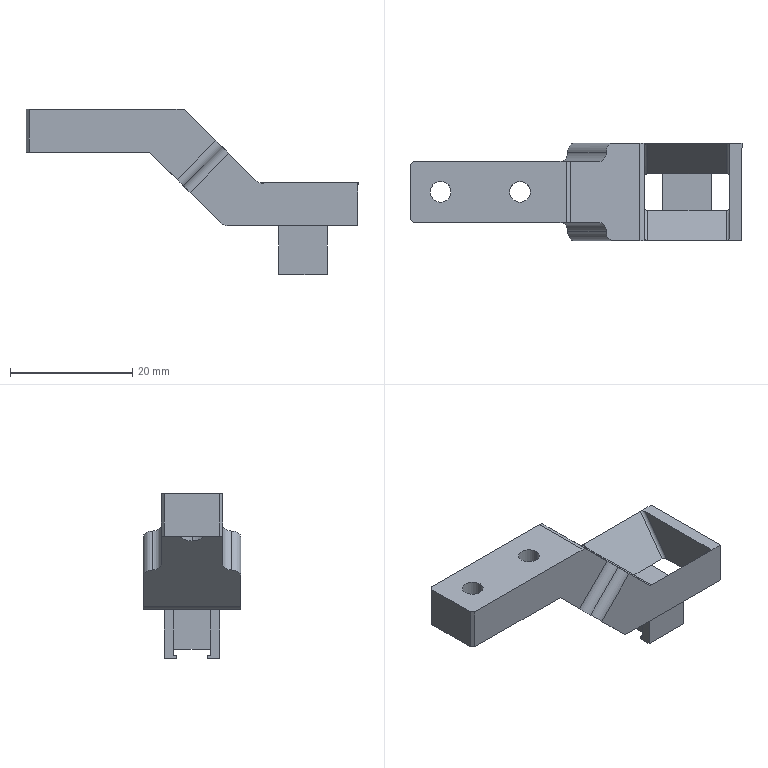NC program | NX | posted with a generic post | part box 54.3 x 16 x 27 mm
Lines 578 to 2261 of 2261, first 1553 of 1680 lines:
(ZLEVEL_PROFILE_COPY_1 , TOOL : D4R0.2)
N1124 T05 M6
N1126 G54
N1128 G17 G0 G90 X3.006 Y-8.122 S9500 M3
N1130 G43 Z30. H5
N1132 Z-4.367
N1134 G94 G1 Z-5.867 F800.
N1136 X3.412 Y-7.653
N1138 G3 X3.488 Y-7.26 R0.4
N1140 G1 X3.424 Y-7.076 F2000.
N1142 X3.414 Y-7.041
N1144 X3.408 Y-7.007
N1146 X3.344 Y-7.003
N1148 X2.618 Y-6.999
N1150 X2.546 Z-5.939
N1152 X3.334 Y-7.007
N1154 X3.344 Y-7.015
N1156 X3.374 Y-7.116
N1158 G3 X3.697 Y-7.893 R3.536
N1160 G1 X3.738 Y-8.01 Z-5.957
N1162 X3.783 Y-8.126 Z-5.975
N1164 X3.834 Y-8.237 Z-5.993
N1166 X3.895 Y-8.343 Z-6.011
N1168 G2 X3.272 Y-7.007 R4.174
N1170 G1 X2.475 Y-6.999
N1172 X2.403 Z-6.083
N1174 X3.062 Y-7.001
N1176 X3.21 Y-7.008
N1178 G3 X4.138 Y-8.696 R3.428
N1180 G1 X4.203 Y-8.795 Z-6.107
N1182 X4.274 Y-8.888 Z-6.131
N1184 X4.356 Y-8.965 Z-6.155
N1186 G2 X3.937 Y-8.559 R1.89
N1188 X3.133 Y-7.008 R3.073
N1190 G1 X3.062 Y-7.003
N1192 X2.332 Y-6.999
N1194 X2.26 Z-6.227
N1196 X3.054 Y-7.007
N1198 G3 X3.344 Y-7.857 R2.478
N1200 X4.534 Y-9.15 R3.612
N1202 G1 X4.62 Y-9.238 Z-6.263
N1204 X4.712 Y-9.319 Z-6.299
N1206 X4.188 Y-8.968
N1208 X3.625 Y-8.431
N1210 G2 X2.983 Y-7.007 R2.952
N1212 G1 X2.188 Y-6.999
N1214 X2.116 Z-6.372
N1216 X2.781 Y-7.001
N1218 X2.911 Y-7.007
N1220 G3 X4.47 Y-9.211 R3.089
N1222 X4.888 Y-9.452 R1.808
N1224 G1 X4.974 Y-9.51 Z-6.408
N1226 X5.062 Y-9.563 Z-6.444
N1228 G2 X4.47 Y-9.263 R2.457
N1230 X3.048 Y-7.717 R3.108
N1232 X2.839 Y-7.007 R2.131
N1234 G1 X2.781 Y-7.003
N1236 X2.045 Y-6.999
N1238 X1.973 Z-6.516
N1240 X2.768 Y-7.007
N1242 X2.86 Y-7.437
N1244 G3 X3.907 Y-8.962 R3.559
N1246 X5.245 Y-9.672 R4.83
N1248 G1 X5.317 Y-9.713 Z-6.552
N1250 X5.393 Y-9.742 Z-6.588
N1252 G2 X5.033 Y-9.621 R1.685
N1254 X3.209 Y-8.279 R3.654
N1256 X2.696 Y-7.007 R3.13
N1258 G1 X1.901 Y-6.999
N1260 X1.83 Z-6.66
N1262 X2.499 Y-7.001
N1264 X2.624 Y-7.007
N1266 G3 X3.137 Y-8.279 R3.13
N1268 X4.47 Y-9.434 R3.933
N1270 X5.556 Y-9.805 R5.388
N1272 G1 X5.636 Y-9.836 Z-6.696
N1274 X5.718 Y-9.859 Z-6.732
N1276 G2 X4.47 Y-9.476 R5.198
N1278 X3.065 Y-8.279 R3.992
N1280 X2.552 Y-7.007 R3.13
N1282 G1 X2.499 Y-7.003
N1284 X1.758 Y-6.999
N1286 X1.686 Z-6.804
N1288 X2.481 Y-7.007
N1290 G3 X2.615 Y-7.537 R1.901
N1292 G1 X2.69 Y-7.717
N1294 G3 X3.834 Y-9.121 R3.339
N1296 X5.314 Y-9.8 R3.733
N1298 G1 X5.88 Y-9.913
N1300 X5.959 Y-9.933 Z-6.84
N1302 X6.04 Y-9.947 Z-6.876
N1304 G2 X5.033 Y-9.761 R9.057
N1306 X3.625 Y-9.021 R4.203
N1308 X2.618 Y-7.717 R3.38
N1310 G1 X2.543 Y-7.537
N1312 G2 X2.409 Y-7.007 R1.901
N1314 G1 X1.615 Y-6.999
N1316 X1.543 Z-6.948
N1318 X2.218 Y-7.001
N1320 X2.337 Y-7.007
N1322 G3 X2.85 Y-8.279 R3.13
N1324 X4.107 Y-9.401 R4.076
N1326 G1 X4.717 Y-9.682
N1328 X4.751 Y-9.694
N1330 G3 X6.203 Y-9.978 R6.263
N1332 G1 X6.282 Y-9.989 Z-6.984
N1334 X6.361 Y-9.997 Z-7.021
N1336 G2 X4.751 Y-9.721 R6.24
N1338 G1 X4.645 Y-9.682
N1340 X4.035 Y-9.401
N1342 G2 X2.779 Y-8.279 R4.076
N1344 X2.266 Y-7.007 R3.13
N1346 G1 X2.218 Y-7.004
N1348 X1.471 Y-6.999
N1350 X1.399 Z-7.093
N1352 X2.194 Y-7.007
N1354 G3 X2.707 Y-8.279 R3.13
N1356 X3.964 Y-9.401 R4.069
N1358 X4.751 Y-9.747 R9.134
N1360 X6.537 Y-9.997 R5.887
N1362 G1 X6.607 Z-7.165
N1364 G2 X5.314 Y-9.908 R6.767
N1366 X4.502 Y-9.682 R6.269
N1368 X2.635 Y-8.279 R4.026
N1370 X2.122 Y-7.007 R3.13
N1372 G1 X1.328 Y-6.999
N1374 X1.256 Z-7.237
N1376 X1.936 Y-7.001
N1378 X2.051 Y-7.007
N1380 G3 X2.563 Y-8.279 R3.13
N1382 X4.58 Y-9.731 R4.005
N1384 G1 X4.751 Y-9.786
N1386 G3 X6.006 Y-9.992 R4.791
N1388 X6.678 Y-9.998 R15.918
N1390 G1 X6.721 Z-7.309
N1392 X5.978 Y-9.995
N1394 X5.925 Y-9.994
N1396 G2 X4.751 Y-9.805 R4.737
N1398 G1 X4.47 Y-9.723
N1400 G2 X2.492 Y-8.279 R4.049
N1402 X1.979 Y-7.007 R3.13
N1404 G1 X1.936 Y-7.004
N1406 X1.184 Y-6.999
N1408 X1.113 Z-7.381
N1410 X1.907 Y-7.007
N1412 G3 X2.42 Y-8.279 R3.13
N1414 X4.751 Y-9.824 R4.048
N1416 X5.925 Y-9.997 R4.658
N1418 G1 X6.721 Y-9.998
N1420 X6.695 Y-9.999 Z-7.453
N1422 X6.028 Y-9.997
N1424 X6.018 Y-10.
N1426 X5.978
N1428 G2 X4.47 Y-9.769 R5.293
N1430 X2.348 Y-8.279 R4.055
N1432 X1.835 Y-7.007 R3.13
N1434 G1 X1.041 Y-6.999
N1436 X0.969 Z-7.525
N1438 X1.655 Y-7.001
N1440 X1.764 Y-7.007
N1442 G3 X2.277 Y-8.279 R3.13
N1444 X4.3 Y-9.734 R4.007
N1446 G1 X4.47 Y-9.788
N1448 G3 X5.925 Y-10. R5.081
N1450 G1 X6.018
N1452 X6.028 Y-9.997
N1454 X6.625 Y-9.999
N1456 X6.554 Z-7.597
N1458 X6.018 Y-10.
N1460 X5.925
N1462 G2 X4.47 Y-9.806 R5.038
N1464 G1 X4.188 Y-9.725
N1466 G2 X2.205 Y-8.279 R4.05
N1468 X1.692 Y-7.007 R3.13
N1470 G1 X1.655 Y-7.004
N1472 X0.897 Y-6.999
N1474 X0.826 Z-7.669
N1476 X1.62 Y-7.007
N1478 G3 X2.262 Y-8.434 R2.938
N1480 G1 X2.366 Y-8.559
N1482 X2.621 Y-8.84
N1484 G3 X4.188 Y-9.751 R4.332
N1486 G1 X4.47 Y-9.825
N1488 G3 X5.925 Y-10. R5.03
N1490 G1 X6.018
N1492 X6.028 Y-9.998
N1494 X6.484 Y-9.999
N1496 X6.414 Z-7.742
N1498 X6.028 Y-9.998
N1500 X6.018 Y-10.
N1502 X5.925
N1504 G2 X4.188 Y-9.77 R5.451
N1506 X2.062 Y-8.279 R4.054
N1508 X1.549 Y-7.007 R3.13
N1510 G1 X1.373 Y-7.001
N1512 X0.67 Y-6.999
N1514 Z-7.814
N1516 X1.373 Y-7.001
N1518 X1.477 Y-7.007
N1520 G3 X1.99 Y-8.279 R3.13
N1522 X4.284 Y-9.812 R4.023
N1524 G1 X4.751 Y-9.926
N1526 G3 X5.925 Y-10. R6.899
N1528 G1 X6.018
N1530 X6.028 Y-9.998
N1532 X6.326 Y-9.999
N1534 X6.255 Z-7.886
N1536 X6.018 Y-10.
N1538 X5.925
N1540 X5.405 Y-9.992
N1542 G2 X4.188 Y-9.808 R4.529
N1544 X1.918 Y-8.279 R4.045
N1546 X1.405 Y-7.007 R3.13
N1548 G1 X1.373 Y-7.004
N1550 X0.67 Y-6.999
N1552 Z-7.958
N1554 X1.334 Y-7.007
N1556 G3 X1.846 Y-8.279 R3.13
N1558 X4.188 Y-9.826 R4.047
N1560 X5.314 Y-9.995 R4.587
N1562 G1 X5.877 Y-9.998
N1564 X5.925 Y-10.
N1566 X6.018
N1568 X6.028 Y-9.998
N1570 X6.185 Y-9.999
N1572 X6.118 Z-8.03
N1574 X6.028 Y-9.998
N1576 X6.018 Y-10.
N1578 X5.925
N1580 G2 X4.801 Y-9.962 R8.862
N1582 X3.907 Y-9.771 R5.87
N1584 X1.775 Y-8.279 R4.053
N1586 X1.262 Y-7.007 R3.13
N1588 G1 X0.467 Y-6.999
N1590 X0.396 Z-8.102
N1592 X1.092 Y-7.001
N1594 X1.19 Y-7.007
N1596 G3 X1.703 Y-8.279 R3.13
N1598 X3.741 Y-9.739 R4.01
N1600 G1 X3.907 Y-9.79
N1602 G3 X5.033 Y-9.988 R4.731
N1604 X5.925 Y-10. R17.353
N1606 G1 X6.018
N1608 X6.037 Y-9.999
N1610 X5.925 Y-10. Z-8.174
N1612 X5.877 Y-9.998
N1614 X5.314 Y-9.997
N1616 G2 X3.907 Y-9.809 R4.825
N1618 G1 X3.766 Y-9.769
N1620 G2 X1.631 Y-8.279 R4.017
N1622 X1.118 Y-7.007 R3.13
N1624 G1 X1.092 Y-7.005
N1626 X0.324 Y-6.999
N1628 X0.252 Z-8.246
N1630 X1.047 Y-7.007
N1632 G3 X1.56 Y-8.279 R3.13
N1634 X3.907 Y-9.828 R4.05
N1636 X5.033 Y-9.995 R4.593
N1638 G1 X5.877 Y-10.
N1640 X5.736 Z-8.282
N1642 X5.596 Z-8.318
N1644 G2 X4.514 Y-9.962 R8.506
N1646 X3.625 Y-9.773 R5.825
N1648 X1.488 Y-8.279 R4.052
N1650 X0.975 Y-7.007 R3.13
N1652 G1 X0.81 Y-7.001
N1654 X0.107 Y-6.999
N1656 Z-8.391
N1658 X0.81 Y-7.002
N1660 X0.903 Y-7.007
N1662 G3 X1.416 Y-8.279 R3.13
N1664 X3.625 Y-9.792 R4.045
N1666 X4.882 Y-9.99 R4.488
N1668 G1 X5.596 Y-10.
N1670 Z-8.463
N1672 X4.85 Y-9.993
N1674 G2 X3.625 Y-9.811 R4.503
N1676 X1.344 Y-8.279 R4.045
N1678 X0.832 Y-7.007 R3.13
N1680 G1 X0.81 Y-7.005
N1682 X0.107 Y-6.999
N1684 X-0.035 Z-8.535
N1686 X0.76 Y-7.007
N1688 G3 X1.273 Y-8.279 R3.13
N1690 X3.625 Y-9.829 R4.051
N1692 X4.751 Y-9.995 R4.599
N1694 G1 X5.596 Y-10.
N1696 X5.455 Z-8.571
N1698 X5.314 Z-8.607
N1700 G2 X4.227 Y-9.962 R8.621
N1702 X3.344 Y-9.774 R5.763
N1704 X1.201 Y-8.279 R4.051
N1706 X0.688 Y-7.007 R3.13
N1708 G1 X-0.106 Y-6.999
N1710 X-0.178 Z-8.679
N1712 X0.529 Y-7.002
N1714 X0.617 Y-7.007
N1716 G3 X1.129 Y-8.279 R3.13
N1718 X3.344 Y-9.793 R4.045
N1720 X4.598 Y-9.99 R4.489
N1722 G1 X5.314 Y-10.
N1724 Z-8.751
N1726 X4.566 Y-9.993
N1728 G2 X3.344 Y-9.812 R4.505
N1730 X1.058 Y-8.279 R4.045
N1732 X0.545 Y-7.007 R3.13
N1734 G1 X-0.25 Y-7.
N1736 X-0.353 Z-8.787
N1738 X-0.456 Z-8.823
N1740 X0.473 Y-7.007
N1742 G3 X0.986 Y-8.279 R3.13
N1744 X3.344 Y-9.83 R4.053
N1746 X4.47 Y-9.996 R4.606
N1748 G1 X5.314 Y-10.
N1750 X5.173 Z-8.859
N1752 X5.033 Z-8.895
N1754 G2 X3.941 Y-9.962 R8.736
N1756 X3.062 Y-9.776 R5.701
N1758 X0.914 Y-8.279 R4.05
N1760 X0.401 Y-7.007 R3.13
N1762 G1 X0.247 Y-7.001
N1764 X-0.456 Y-7.
N1766 Z-8.967
N1768 X0.247 Y-7.002
N1770 X0.33 Y-7.007
N1772 G3 X0.843 Y-8.279 R3.13
N1774 X3.062 Y-9.795 R4.044
N1776 X4.314 Y-9.99 R4.49
N1778 G1 X5.033 Y-10.
N1780 Z-9.04
N1782 X4.282 Y-9.993
N1784 G2 X3.062 Y-9.813 R4.506
N1786 X0.771 Y-8.279 R4.045
N1788 X0.258 Y-7.008 R3.13
N1790 G1 X0.212 Y-7.003
N1792 X-0.456 Y-7.
N1794 X-0.532 Z-9.076
N1796 X-0.608 Z-9.112
N1798 X0.14 Y-7.003
N1800 X0.186 Y-7.006
N1802 G3 X0.699 Y-8.279 R3.13
N1804 X3.062 Y-9.832 R4.054
N1806 X4.014 Y-9.988 R4.474
N1808 X5.033 Y-10. R11.986
N1810 G1 X4.892 Z-9.148
N1812 X4.751 Z-9.184
N1814 G2 X3.654 Y-9.962 R8.85
N1816 X2.781 Y-9.777 R5.637
N1818 X0.627 Y-8.279 R4.05
N1820 X0.114 Y-7.006 R3.13
N1822 G1 X-0.034 Y-7.001
N1824 X-0.68 Y-6.999
N1826 X-0.752 Z-9.256
N1828 X-0.034 Y-7.002
N1830 X0.043 Y-7.006
N1832 G3 X0.556 Y-8.279 R3.13
N1834 X2.781 Y-9.796 R4.044
N1836 X4.03 Y-9.99 R4.491
N1838 G1 X4.751 Y-10.
N1840 Z-9.328
N1842 X3.998 Y-9.993
N1844 G2 X2.781 Y-9.815 R4.508
N1846 X0.484 Y-8.279 R4.045
N1848 X-0.029 Y-7.009 R3.13
N1850 G1 X-0.06 Y-7.004
N1852 X-0.823 Y-6.998
N1854 X-0.921 Y-7. Z-9.364
N1856 X-1.019 Y-6.998 Z-9.4
N1858 X-0.101 Y-7.006
N1860 G3 X0.412 Y-8.279 R3.13
N1862 X2.781 Y-9.833 R4.054
N1864 X3.907 Y-9.996 R4.62
N1866 G1 X4.47 Y-10.
N1868 Z-9.472
N1870 G2 X3.658 Y-9.986 R8.963
N1872 X2.223 Y-9.687 R5.187
N1874 X0.341 Y-8.279 R4.031
N1876 X-0.172 Y-7.006 R3.13
N1878 G1 X-0.315 Y-7.
N1880 X-1.019 Y-6.999
N1882 Z-9.544
N1884 X-0.315 Y-7.002
N1886 X-0.244 Y-7.006
N1888 G3 X0.269 Y-8.279 R3.13
N1890 X2.499 Y-9.797 R4.044
N1892 X3.747 Y-9.991 R4.492
N1894 G1 X4.47 Y-10.
N1896 Z-9.616
N1898 X3.714 Y-9.994
N1900 G2 X2.499 Y-9.816 R4.509
N1902 X0.197 Y-8.279 R4.046
N1904 X-0.316 Y-7.007 R3.142
N1906 G1 X-0.34 Y-7.005
N1908 X-1.019 Y-6.999
N1910 X-1.101 Y-7. Z-9.652
N1912 X-1.182 Y-6.999 Z-9.689
N1914 X-0.387 Y-7.007
N1916 G3 X0.126 Y-8.279 R3.13
N1918 X2.499 Y-9.834 R4.055
N1920 X3.625 Y-9.997 R4.628
N1922 G1 X4.188 Y-10.
N1924 Z-9.761
N1926 G2 X3.371 Y-9.985 R9.064
N1928 X1.936 Y-9.687 R5.182
N1930 X0.054 Y-8.279 R4.032
N1932 X-0.459 Y-7.007 R3.13
N1934 G1 X-0.597 Y-7.
N1936 X-1.254 Y-6.999
N1938 X-1.325 Y-7. Z-9.833
N1940 X-0.597 Y-7.003
N1942 X-0.531 Y-7.007
N1944 G3 X-0.018 Y-8.279 R3.13
N1946 X2.218 Y-9.799 R4.044
N1948 X3.463 Y-9.991 R4.493
N1950 G1 X4.188 Y-10.
N1952 Z-9.905
N1954 X3.43 Y-9.994
N1956 G2 X2.218 Y-9.818 R4.511
N1958 X-0.09 Y-8.279 R4.046
N1960 X-0.603 Y-7.007 R3.13
N1962 G1 X-1.397 Y-7.
N1964 X-1.506 Z-9.929
N1966 X-1.614 Z-9.953
N1968 X-1.723 Z-9.977
N1970 X-0.878
N1972 X-0.674 Y-7.007
N1974 G3 X-0.033 Y-8.434 R2.938
N1976 G1 X0.071 Y-8.559
N1978 X0.327 Y-8.84
N1980 G3 X1.936 Y-9.762 R4.297
N1982 G1 X2.218 Y-9.836
N1984 G3 X3.907 Y-10. R5.688
N1986 G1 Z-10.049
N1988 G2 X3.094 Y-9.986 R9.188
N1990 X1.664 Y-9.693 R5.207
N1992 X-0.233 Y-8.279 R4.032
N1994 X-0.746 Y-7.007 R3.13
N1996 G1 X-0.878 Y-7.
N1998 X-1.723
N2000 Z-10.121
N2002 X-0.878 Y-7.003
N2004 X-0.818 Y-7.007
N2006 G3 X-0.305 Y-8.279 R3.13
N2008 X1.936 Y-9.8 R4.044
N2010 X3.179 Y-9.991 R4.495
N2012 G1 X3.907 Y-10.
N2014 Z-10.193
N2016 X3.146 Y-9.994
N2018 G2 X1.936 Y-9.819 R4.512
N2020 X-0.376 Y-8.279 R4.046
N2022 X-0.889 Y-7.007 R3.13
N2024 G1 X-1.723 Y-7.
N2026 X-2.004 Z-10.265
N2028 X-1.16 Y-7.001
N2030 X-0.961 Y-7.007
N2032 G3 X-0.827 Y-7.537 R1.902
N2034 G1 X-0.752 Y-7.717
N2036 G3 X0.348 Y-9.088 R3.343
N2038 G1 X0.392 Y-9.121
N2040 G3 X1.655 Y-9.764 R3.942
N2042 X3.625 Y-10. R5.868
N2044 G1 Z-10.337
N2046 X3.062 Y-9.997
N2048 G2 X1.655 Y-9.783 R4.973
N2050 G1 X1.482 Y-9.727
N2052 G2 X-0.52 Y-8.279 R4.01
N2054 X-1.033 Y-7.007 R3.13
N2056 G1 X-1.16 Y-7.001
N2058 X-2.004 Y-7.
N2060 Z-10.41
N2062 X-1.16 Y-7.003
N2064 X-1.104 Y-7.007
N2066 G3 X-0.592 Y-8.279 R3.13
N2068 X1.655 Y-9.802 R4.045
N2070 X2.895 Y-9.991 R4.496
N2072 G1 X3.625 Y-10.
N2074 Z-10.482
N2076 X2.781 Y-9.994
N2078 G2 X1.655 Y-9.82 R4.585
N2080 X-0.663 Y-8.279 R4.047
N2082 X-1.176 Y-7.007 R3.13
N2084 G1 X-2.004 Y-7.
N2086 X-2.286 Z-10.554
N2088 X-1.441
N2090 X-1.248 Y-7.007
N2092 G3 X-0.735 Y-8.279 R3.13
N2094 X1.373 Y-9.765 R4.058
N2096 X3.344 Y-10. R5.878
N2098 G1 Z-10.626
N2100 X2.781 Y-9.997
N2102 G2 X1.373 Y-9.784 R4.951
N2104 G1 X1.202 Y-9.729
N2106 G2 X-0.807 Y-8.279 R4.012
N2108 X-1.319 Y-7.007 R3.13
N2110 G1 X-1.441 Y-7.
N2112 X-2.286
N2114 Z-10.698
N2116 X-1.441 Y-7.003
N2118 X-1.391 Y-7.007
N2120 G3 X-0.878 Y-8.279 R3.13
N2122 X1.373 Y-9.803 R4.045
N2124 X2.611 Y-9.992 R4.497
N2126 G1 X3.344 Y-10.
N2128 Z-10.77
N2130 X2.499 Y-9.994
N2132 G2 X1.373 Y-9.822 R4.58
N2134 X-0.95 Y-8.279 R4.047
N2136 X-1.463 Y-7.008 R3.131
N2138 G1 X-2.286 Y-7.
N2140 X-2.567 Z-10.842
N2142 X-1.723
N2144 X-1.534 Y-7.008
N2146 G3 X-1.022 Y-8.279 R3.13
N2148 X1.092 Y-9.767 R4.057
N2150 X3.062 Y-10. R5.902
N2152 G1 Z-10.914
N2154 X2.499 Y-9.997
N2156 G2 X1.092 Y-9.785 R4.932
N2158 G1 X0.92 Y-9.73
N2160 G2 X-1.093 Y-8.279 R4.004
N2162 X-1.606 Y-7.008 R3.13
N2164 G1 X-1.723 Y-7.001
N2166 X-2.567 Y-7.
N2168 Z-10.986
N2170 X-1.723 Y-7.004
N2172 X-1.678 Y-7.008
N2174 G3 X-1.165 Y-8.279 R3.13
N2176 X1.092 Y-9.804 R4.045
N2178 X2.327 Y-9.992 R4.498
N2180 G1 X3.062 Y-10.
N2182 Z-11.059
N2184 X2.218 Y-9.994
N2186 G2 X1.092 Y-9.823 R4.573
N2188 X-1.237 Y-8.279 R4.047
N2190 X-1.75 Y-7.008 R3.13
N2192 G1 X-2.567 Y-7.
N2194 X-2.708 Z-11.131
N2196 X-2.567
N2198 X-1.821 Y-7.008
N2200 G3 X-1.309 Y-8.279 R3.13
N2202 X0.81 Y-9.768 R4.056
N2204 X2.781 Y-10. R5.934
N2206 G1 Z-11.203
N2208 X2.218 Y-9.997
N2210 G2 X0.81 Y-9.787 R4.913
N2212 G1 X0.64 Y-9.733
N2214 G2 X-1.38 Y-8.279 R4.006
N2216 X-1.893 Y-7.008 R3.13
N2218 G1 X-2.004 Y-7.001
N2220 X-2.708 Y-7.
N2222 Z-11.275
N2224 X-2.004 Y-7.005
N2226 X-1.965 Y-7.008
N2228 G3 X-1.452 Y-8.279 R3.13
N2230 X0.81 Y-9.806 R4.045
N2232 X2.043 Y-9.992 R4.499
N2234 G1 X2.781 Y-10.
N2236 Z-11.347
N2238 X1.936 Y-9.995
N2240 G2 X0.81 Y-9.824 R4.579
N2242 X-1.524 Y-8.279 R4.046
N2244 X-2.036 Y-7.009 R3.131
N2246 G1 X-2.708 Y-7.
N2248 X-2.806 Z-11.383
N2250 X-2.905 Z-11.419
N2252 G2 X-2.108 Y-7.009 R17.77
N2254 G3 X-1.595 Y-8.279 R3.131
N2256 X0.529 Y-9.769 R4.054
N2258 X1.431 Y-9.962 R5.957
N2260 X2.499 Y-10. R8.221
N2262 G1 Z-11.491
N2264 G2 X1.655 Y-9.987 R14.64
N2266 X0.529 Y-9.788 R4.78
N2268 G1 X0.361 Y-9.735
N2270 G2 X-1.667 Y-8.279 R4.008
N2272 X-2.18 Y-7.009 R3.131
N2274 G1 X-2.286 Y-7.001
N2276 X-2.969 Y-7.
N2278 X-3.05 Z-11.563
N2280 X-2.352 Y-7.001
N2282 X-2.251 Y-7.009
N2284 G3 X-1.739 Y-8.279 R3.131
N2286 X0.529 Y-9.807 R4.045
N2288 X1.759 Y-9.992 R4.501
N2290 G1 X2.499 Y-10.
N2292 Z-11.635
N2294 X1.655 Y-9.995
N2296 G2 X0.529 Y-9.826 R4.584
N2298 X-1.81 Y-8.279 R4.047
N2300 X-2.324 Y-7.003 R3.13
N2302 G1 X-2.423 Y-7.001
N2304 X-3.058 Y-7.
N2306 X-3.124
N2308 X-3.099 Z-11.708
N2310 X-3.042
N2312 X-2.493 Y-7.001
N2314 X-2.396 Y-7.004
N2316 G3 X-1.882 Y-8.279 R3.129
N2318 X0.247 Y-9.771 R4.053
N2320 X1.144 Y-9.962 R5.897
N2322 X2.218 Y-10. R8.338
N2324 G1 Z-11.78
N2326 G2 X1.373 Y-9.988 R15.127
N2328 X0.247 Y-9.79 R4.747
N2330 G1 X0.081 Y-9.737
N2332 G2 X-1.954 Y-8.279 R4.009
N2334 X-2.467 Y-7.004 R3.13
N2336 G1 X-2.567 Y-7.001
N2338 X-3.034 Y-7.
N2340 X-2.953 Z-11.852
N2342 X-2.538 Y-7.012
N2344 G3 X-2.026 Y-8.279 R3.132
N2346 X0.247 Y-9.809 R4.045
N2348 X1.475 Y-9.992 R4.502
N2350 G1 X2.218 Y-10.
N2352 Z-11.924
N2354 X1.373 Y-9.995
N2356 G2 X0.247 Y-9.827 R4.59
N2358 X-2.097 Y-8.279 R4.049
N2360 X-2.609 Y-7.017 R3.135
N2362 G1 X-2.888 Y-7.
N2364 X-2.801 Y-7.009 Z-11.996
N2366 X-2.679 Y-7.026
N2368 G3 X-2.169 Y-8.279 R3.141
N2370 X-0.034 Y-9.772 R4.052
N2372 X0.857 Y-9.962 R5.837
N2374 X1.936 Y-10. R8.455
N2376 G1 Z-12.068
N2378 G2 X1.092 Y-9.988 R15.649
N2380 X-0.034 Y-9.791 R4.725
N2382 G1 X-0.198 Y-9.74
N2384 G2 X-2.241 Y-8.279 R4.011
N2386 X-2.749 Y-7.036 R3.15
N2388 G1 X-2.825 Y-7.02
N2390 X-2.857 Y-7.034 Z-12.14
N2392 X-2.82 Y-7.04
N2394 G3 X-2.312 Y-8.279 R3.151
N2396 X-0.034 Y-9.81 R4.045
N2398 X1.192 Y-9.993 R4.503
N2400 G1 X1.936 Y-10.
N2402 Z-12.212
N2404 X1.092 Y-9.995
N2406 G2 X-0.034 Y-9.828 R4.596
N2408 X-2.384 Y-8.279 R4.05
N2410 X-2.891 Y-7.048 R3.179
N2412 G1 X-2.963 Y-7.049 Z-12.284
N2414 G3 X-2.456 Y-8.279 R3.183
N2416 X-0.315 Y-9.774 R4.052
N2418 X0.571 Y-9.962 R5.792
N2420 X1.655 Y-10. R8.568
N2422 G1 Z-12.356
N2424 X0.94 Y-9.99
N2426 G2 X-0.315 Y-9.792 R4.488
N2428 X-2.527 Y-8.279 R4.045
N2430 X-3.035 Y-7.045 R3.17
N2432 G1 X-3.113 Y-7.034 Z-12.429
N2434 X-3.108 Y-7.036
N2436 X-3.019 Y-7.437
N2438 G3 X-2.599 Y-8.279 R4.703
N2440 X-0.315 Y-9.811 R4.044
N2442 X0.908 Y-9.993 R4.504
N2444 G1 X1.655 Y-10.
N2446 Z-12.501
N2448 X0.81 Y-9.996
N2450 G2 X-0.315 Y-9.83 R4.603
N2452 X-1.83 Y-9.121 R3.932
N2454 G1 X-2.004 Y-8.994
N2456 G2 X-2.971 Y-7.717 R3.379
N2458 G1 X-3.046 Y-7.543
N2460 G2 X-3.181 Y-7.025 R1.824
N2462 G1 X-3.258 Y-7.006 Z-12.573
N2464 G3 X-2.658 Y-8.388 R3.174
N2466 X-0.597 Y-9.775 R4.029
N2468 X0.284 Y-9.962 R5.729
N2470 X1.373 Y-10. R8.684
N2472 G1 Z-12.645
N2474 X0.656 Y-9.99
N2476 G2 X-0.597 Y-9.794 R4.489
N2478 X-2.814 Y-8.279 R4.045
N2480 X-3.326 Y-7. R3.402
N2482 G1 X-3.396 Z-12.717
N2484 G3 X-2.398 Y-8.84 R3.461
N2486 X-1.629 Y-9.401 R6.035
N2488 X0.658 Y-9.993 R4.886
N2490 G1 X1.373 Y-10.
N2492 Z-12.789
N2494 X0.529 Y-9.996
N2496 G2 X-0.597 Y-9.831 R4.61
N2498 X-2.567 Y-8.737 R4.107
N2500 X-3.451 Y-7. R3.594
N2502 G1 X-3.514 Z-12.861
N2504 G3 X-2.526 Y-8.84 R3.752
N2506 X-1.772 Y-9.401 R4.885
N2508 G1 X-1.723 Y-9.425
N2510 X-1.163 Y-9.682
N2512 G3 X-0.003 Y-9.962 R5.528
N2514 X1.092 Y-10. R8.797
N2516 G1 Z-12.933
N2518 G2 X0.193 Y-9.983 R10.875
N2520 X-1.234 Y-9.682 R4.941
N2522 G1 X-1.844 Y-9.401
N2524 G2 X-2.585 Y-8.84 R4.447
N2526 G1 X-3.046 Y-8.279
N2528 G2 X-3.589 Y-7. R4.043
N2530 G1 X-3.565 Y-7.117 Z-12.945
N2532 X-3.546 Y-7.235 Z-12.958
N2534 X-3.526 Y-7.354 Z-12.97
N2536 X-3.5 Y-7.471 Z-12.982
N2538 X-3.468 Y-7.585 Z-12.994
N2540 X-3.427 Y-7.696 Z-13.006
N2542 X-3.418 Y-7.717
N2544 X-3.283 Y-7.998
N2546 G3 X-2.004 Y-9.349 R4.09
N2548 X0.247 Y-9.992 R4.878
N2550 G1 X1.092 Y-10.
N2552 X0.951 Z-13.045
N2554 X0.81 Z-13.084
N2556 X0.247 Y-9.996
N2558 G2 X-0.878 Y-9.834 R4.625
N2560 X-2.004 Y-9.383 R4.095
N2562 X-3.17 Y-8.3 R4.651
N2564 G1 X-3.109 Y-8.401 Z-13.104
N2566 X-3.045 Y-8.499 Z-13.124
N2568 X-2.98 Y-8.596 Z-13.144
N2570 X-2.913 Y-8.691 Z-13.165
N2572 G3 X-2.413 Y-9.121 R2.421
N2574 X-0.878 Y-9.854 R3.522
N2576 X-0.034 Y-9.986 R3.981
N2578 X0.81 Y-10. R12.728
N2580 G1 Z-13.249
N2582 G2 X-0.083 Y-9.985 R12.379
N2584 X-1.441 Y-9.722 R4.985
N2586 X-2.673 Y-8.982 R4.922
N2588 G1 X-2.6 Y-9.066 Z-13.278
N2590 X-2.521 Y-9.144 Z-13.308
N2592 X-2.439 Y-9.217 Z-13.337
N2594 G3 X-2.004 Y-9.472 R2.042
N2596 X-1.345 Y-9.769 R2.77
N2598 G1 X-1.16 Y-9.824
N2600 G3 X-0.034 Y-9.995 R4.441
N2602 G1 X0.81 Y-10.
N2604 X0.67 Z-13.382
N2606 X0.529 Z-13.427
N2608 X-0.059 Y-9.997
N2610 G2 X-1.475 Y-9.741 R4.143
N2612 G1 X-1.723 Y-9.65
N2614 X-2.004 Y-9.511
N2616 X-2.208 Y-9.415
N2618 X-2.098 Y-9.489 Z-13.474
N2620 X-1.986 Y-9.56 Z-13.52
N2622 G3 X-1.441 Y-9.771 R3.272
N2624 X-0.315 Y-9.99 R3.412
N2626 X0.529 Y-10. R26.
N2628 G1 Z-13.615
N2630 G2 X-0.597 Y-9.981 R19.801
N2632 X-1.763 Y-9.693 R5.316
N2634 G1 X-1.656 Y-9.742 Z-13.664
N2636 X-1.547 Y-9.785 Z-13.712
N2638 G3 X-0.315 Y-9.998 R3.988
N2640 G1 X0.247 Y-10.
N2642 Z-13.806
N2644 G2 X-0.597 Y-9.985 R14.095
N2646 X-1.342 Y-9.868 R3.695
N2648 G1 X-1.244 Y-9.901 Z-13.837
N2650 X-1.144 Y-9.924 Z-13.869
N2652 X-1.044 Y-9.944 Z-13.9
N2654 G3 X-0.315 Y-9.998 R4.014
N2656 G1 X0.247 Y-10.
N2658 G2 X0.593 Y-10.201 R0.4
N2660 G1 X0.937 Y-10.8
N2662 Z-12.4
N2664 G0 Z30.
N2666 X1.846 Y7.8
N2668 Z-4.439
N2670 G1 Z-5.939 F800.
N2672 X2.199 Y7.197
N2674 G3 X2.546 Y7. R0.4
N2676 G1 X3.319 Y7.005 F2000.
N2678 X3.378 Y7.017
N2680 G2 X3.674 Y7.841 R2.599
N2682 G1 X3.72 Y7.972 Z-5.957
N2684 X3.769 Y8.102 Z-5.975
N2686 X3.827 Y8.226 Z-5.993
N2688 X3.895 Y8.343 Z-6.011
N2690 G3 X3.29 Y7.009 R3.763
N2692 G1 X3.248 Y7.005
N2694 X2.475 Y7.
N2696 X2.403 Z-6.083
N2698 X3.062
N2700 X3.202 Y7.007
N2702 G2 X4.138 Y8.696 R3.511
N2704 G1 X4.195 Y8.788 Z-6.107
N2706 X4.259 Y8.875 Z-6.131
N2708 X4.333 Y8.947 Z-6.155
N2710 G3 X3.937 Y8.559 R1.869
N2712 X3.127 Y7.007 R3.107
N2714 G1 X3.062 Y7.003
N2716 X2.332 Y7.
N2718 X2.26 Z-6.227
N2720 X3.054 Y7.007
N2722 G2 X3.907 Y8.614 R2.886
N2724 X4.535 Y9.15 R2.545
N2726 G1 X4.621 Y9.239 Z-6.263
N2728 X4.712 Y9.319 Z-6.299
N2730 G3 X3.767 Y8.581 R4.691
N2732 X2.983 Y7.007 R2.817
N2734 G1 X2.965 Y7.005
N2736 X2.188 Y7.
N2738 X2.116 Z-6.372
N2740 X2.781
N2742 X2.911 Y7.007
N2744 G2 X4.47 Y9.211 R3.088
N2746 X4.895 Y9.455 R1.833
N2748 G1 X4.986 Y9.516 Z-6.408
N2750 X5.078 Y9.569 Z-6.444
N2752 G3 X4.47 Y9.263 R2.475
N2754 X3.625 Y8.604 R2.503
N2756 X2.839 Y7.007 R3.007
N2758 G1 X2.781 Y7.003
N2760 X2.045 Y7.
N2762 X1.973 Z-6.516
N2764 X2.768 Y7.007
N2766 G2 X2.902 Y7.536 R1.898
N2768 G1 X2.977 Y7.717
N2770 G2 X4.61 Y9.401 R3.319
N2772 X5.246 Y9.673 R6.973
N2774 G1 X5.326 Y9.716 Z-6.552
N2776 X5.41 Y9.748 Z-6.588
N2778 G3 X4.496 Y9.401 R6.012
N2780 X3.209 Y8.279 R3.774
N2782 X2.696 Y7.007 R3.129
N2784 G1 X2.681 Y7.006
N2786 X1.901 Y7.
N2788 X1.83 Z-6.66
N2790 X2.499
N2792 X2.624 Y7.007
N2794 G2 X3.137 Y8.279 R3.129
N2796 X4.47 Y9.434 R3.924
N2798 X5.604 Y9.823 R6.175
N2800 G1 X5.737 Y9.869 Z-6.732
N2802 G3 X4.47 Y9.476 R5.718
N2804 X3.065 Y8.279 R3.978
N2806 X2.552 Y7.007 R3.129
N2808 G1 X2.499 Y7.003
N2810 X1.758 Y7.
N2812 X1.686 Z-6.804
N2814 X2.481 Y7.007
N2816 G2 X2.683 Y7.701 R2.872
N2818 X3.625 Y8.966 R3.443
N2820 X4.251 Y9.401 R10.279
N2822 X5.227 Y9.777 R4.016
N2824 X5.867 Y9.92 R17.863
N2826 G1 X5.955 Y9.941 Z-6.84
N2828 X6.043 Y9.957 Z-6.876
N2830 G3 X5.033 Y9.761 R11.445
N2832 X3.625 Y9.021 R4.203
N2834 X2.618 Y7.717 R3.38
N2836 G1 X2.543 Y7.536
N2838 G3 X2.409 Y7.007 R1.898
N2840 G1 X2.395 Y7.006
N2842 X1.615 Y7.
N2844 X1.543 Z-6.948
N2846 X2.218 Y7.001
N2848 X2.337 Y7.007
N2850 G2 X2.85 Y8.279 R3.129
N2852 X4.107 Y9.401 R4.076
N2854 G1 X4.717 Y9.682
N2856 X4.751 Y9.694
N2858 G2 X6.203 Y9.982 R6.503
N2860 G1 X6.273 Y9.99 Z-6.984
N2862 X6.343 Y9.998 Z-7.021
N2864 G3 X4.751 Y9.721 R6.497
N2866 G1 X4.645 Y9.682
N2868 X4.035 Y9.401
N2870 G3 X2.779 Y8.279 R4.076
N2872 X2.266 Y7.007 R3.129
N2874 G1 X2.218 Y7.004
N2876 X1.471 Y7.
N2878 X1.399 Z-7.093
N2880 X2.194 Y7.007
N2882 G2 X2.707 Y8.279 R3.129
N2884 X3.964 Y9.401 R4.069
N2886 X4.751 Y9.747 R9.134
N2888 X6.537 Y9.998 R5.985
N2890 G1 X6.607 Z-7.165
N2892 G3 X5.978 Y9.982 R5.286
N2894 G1 X5.943 Y9.981
N2896 X5.877 Y9.978
N2898 G3 X3.892 Y9.401 R4.85
N2900 X2.635 Y8.279 R4.076
N2902 X2.122 Y7.007 R3.129
N2904 G1 X2.108 Y7.006
N2906 X1.328 Y7.
N2908 X1.256 Z-7.237
N2910 X1.936 Y7.001
N2912 X2.051 Y7.007
N2914 G2 X2.563 Y8.279 R3.129
N2916 X4.58 Y9.731 R4.005
N2918 G1 X4.751 Y9.786
N2920 G2 X6.061 Y9.996 R4.958
N2922 G1 X6.11 Y9.997
N2924 X6.669 Y10.
N2926 X6.678 Y9.998
N2928 X6.729 Y10. Z-7.309
N2930 X6.028 Y9.997
N2932 G3 X4.751 Y9.805 R4.777
N2934 G1 X4.47 Y9.723
N2936 G3 X2.492 Y8.279 R4.049
N2938 X1.979 Y7.007 R3.129
N2940 G1 X1.936 Y7.004
N2942 X1.184 Y7.
N2944 X1.113 Z-7.381
N2946 X1.907 Y7.007
N2948 G2 X2.42 Y8.279 R3.129
N2950 X4.751 Y9.824 R4.048
N2952 X6.028 Y9.997 R4.637
N2954 G1 X6.729 Y10.
N2956 X6.695 Z-7.453
N2958 X5.988
N2960 G3 X4.47 Y9.769 R5.289
N2962 X2.348 Y8.279 R4.055
N2964 X1.835 Y7.007 R3.129
N2966 G1 X1.821 Y7.006
N2968 X1.041 Y7.
N2970 X0.969 Z-7.525
N2972 X1.655 Y7.001
N2974 X1.764 Y7.007
N2976 G2 X2.277 Y8.279 R3.129
N2978 X4.3 Y9.734 R4.007
N2980 G1 X4.47 Y9.788
N2982 G2 X5.942 Y10. R5.086
N2984 G1 X6.625
N2986 X6.554 Z-7.597
N2988 X6.028 Y9.998
N2990 X6.018 Y10.
N2992 X5.942
N2994 G3 X4.47 Y9.806 R5.057
N2996 G1 X4.188 Y9.725
N2998 G3 X2.205 Y8.279 R4.05
N3000 X1.692 Y7.007 R3.129
N3002 G1 X0.897 Y7.
N3004 X0.826 Z-7.669
N3006 X1.62 Y7.007
N3008 G2 X2.133 Y8.279 R3.129
N3010 G1 X2.366 Y8.559
N3012 X2.621 Y8.84
N3014 G2 X4.188 Y9.751 R4.332
N3016 G1 X4.47 Y9.825
N3018 G2 X5.942 Y10. R5.062
N3020 G1 X6.018
N3022 X6.028 Y9.998
N3024 X6.484 Y10.
N3026 X6.414 Z-7.742
N3028 X6.028 Y9.999
N3030 X6.018 Y10.
N3032 X5.942
N3034 G3 X4.188 Y9.77 R5.477
N3036 X2.062 Y8.279 R4.054
N3038 X1.549 Y7.007 R3.129
N3040 G1 X1.373 Y7.
N3042 X0.67
N3044 Z-7.814
N3046 X1.373 Y7.001
N3048 X1.477 Y7.007
N3050 G2 X1.99 Y8.279 R3.129
N3052 X4.021 Y9.736 R4.009
N3054 G1 X4.188 Y9.789
N3056 G2 X5.596 Y9.997 R4.897
N3058 G1 X5.877 Y9.998
N3060 X5.942 Y10.
N3062 X6.018
N3064 X6.028 Y9.999
N3066 X6.326 Y10.
N3068 X6.255 Z-7.886
N3070 X6.018
N3072 X5.942
N3074 X5.405 Y9.992
N3076 G3 X4.215 Y9.815 R4.516
N3078 G1 X3.907 Y9.726
N3080 G3 X1.918 Y8.279 R4.052
N3082 X1.405 Y7.007 R3.129
N3084 G1 X0.67 Y7.
N3086 Z-7.958
N3088 X1.334 Y7.007
N3090 G2 X1.846 Y8.279 R3.129
N3092 X4.188 Y9.826 R4.047
N3094 X5.314 Y9.995 R4.587
N3096 G1 X5.942 Y10.
N3098 X6.018
N3100 X6.185
N3102 X6.118 Z-8.03
N3104 X5.942
N3106 X5.877 Y9.999
N3108 X5.381 Y9.997
N3110 G3 X3.794 Y9.733 R5.013
N3112 G1 X3.641 Y9.682
N3114 X3.032 Y9.401
N3116 G3 X1.775 Y8.279 R4.076
N3118 X1.262 Y7.007 R3.129
N3120 G1 X1.248 Y7.006
N3122 X0.467 Y7.
N3124 X0.396 Z-8.102
N3126 X1.092 Y7.001
N3128 X1.19 Y7.007
N3130 G2 X1.703 Y8.279 R3.129
N3132 X3.741 Y9.739 R4.01
N3134 G1 X3.907 Y9.79
N3136 G2 X5.314 Y9.997 R4.881
N3138 G1 X5.942 Y10.
N3140 X6.052
N3142 X5.942 Z-8.174
N3144 X5.134 Y9.992
N3146 G3 X3.94 Y9.819 R4.482
N3148 G1 X3.766 Y9.769
N3150 G3 X1.631 Y8.279 R4.017
N3152 X1.118 Y7.007 R3.129
N3154 G1 X0.324 Y7.
N3156 X0.252 Z-8.246
N3158 X1.032 Y7.006
N3160 X1.047 Y7.007
N3162 G2 X1.56 Y8.279 R3.129
N3164 X2.817 Y9.401 R4.069
N3166 X5.033 Y9.995 R4.949
N3168 G1 X5.877 Y10.
N3170 X5.736 Z-8.282
N3172 X5.596 Z-8.318
N3174 G3 X4.514 Y9.962 R8.479
N3176 X3.625 Y9.773 R5.825
N3178 X1.488 Y8.279 R4.052
N3180 X0.975 Y7.007 R3.129
N3182 G1 X0.81 Y7.
N3184 X0.107
N3186 Z-8.391
N3188 X0.81 Y7.002
N3190 X0.903 Y7.007
N3192 G2 X1.416 Y8.279 R3.129
N3194 X3.462 Y9.741 R4.012
N3196 G1 X3.625 Y9.792
N3198 G2 X4.751 Y9.988 R4.723
N3200 X5.596 Y10. R15.293
N3202 G1 Z-8.463
N3204 X4.848 Y9.993
N3206 G3 X3.662 Y9.821 R4.487
N3208 G1 X3.484 Y9.77
N3210 G3 X1.344 Y8.279 R4.012
N3212 X0.832 Y7.007 R3.129
N3214 G1 X0.107 Y7.
N3216 X-0.035 Z-8.535
N3218 X0.745 Y7.006
N3220 X0.76 Y7.007
N3222 G2 X1.273 Y8.279 R3.129
N3224 X3.625 Y9.829 R4.051
N3226 X4.751 Y9.995 R4.599
N3228 G1 X5.596 Y10.
N3230 X5.455 Z-8.571
N3232 X5.314 Z-8.607
N3234 G3 X4.227 Y9.962 R8.591
N3236 X3.344 Y9.774 R5.763
N3238 X1.201 Y8.279 R4.051
N3240 X0.688 Y7.007 R3.129
N3242 G1 X0.674 Y7.006
N3244 X-0.106 Y7.
N3246 X-0.178 Z-8.679
N3248 X0.529 Y7.002
N3250 X0.617 Y7.007
N3252 G2 X1.129 Y8.279 R3.129
N3254 X3.183 Y9.743 R4.014
N3256 G1 X3.344 Y9.793
N3258 G2 X4.47 Y9.988 R4.717
N3260 X5.314 Y10. R15.795
N3262 G1 Z-8.751
N3264 X4.566 Y9.993
N3266 G3 X3.344 Y9.812 R4.505
N3268 X1.058 Y8.279 R4.045
N3270 X0.545 Y7.007 R3.129
N3272 G1 X-0.25 Y7.
N3274 X-0.353 Z-8.787
N3276 X-0.456 Z-8.823
N3278 X0.459 Y7.006
N3280 X0.473 Y7.007
N3282 G2 X0.986 Y8.279 R3.129
N3284 X3.344 Y9.83 R4.053
N3286 X4.47 Y9.996 R4.606
N3288 G1 X5.314 Y10.
N3290 X5.173 Z-8.859
N3292 X5.033 Z-8.895
N3294 G3 X3.941 Y9.962 R8.702
N3296 X3.062 Y9.776 R5.701
N3298 X0.914 Y8.279 R4.05
N3300 X0.401 Y7.007 R3.129
N3302 G1 X0.247 Y7.
N3304 X-0.456
N3306 Z-8.967
N3308 X0.247 Y7.002
N3310 X0.33 Y7.007
N3312 G2 X0.843 Y8.279 R3.129
N3314 X2.903 Y9.746 R4.015
N3316 G1 X3.057 Y9.793
N3318 G2 X4.313 Y9.99 R4.484
N3320 G1 X5.033 Y10.
N3322 Z-9.04
N3324 X4.282 Y9.993
N3326 G3 X3.062 Y9.813 R4.506
N3328 X0.771 Y8.279 R4.045
N3330 X0.258 Y7.008 R3.129
N3332 G1 X0.215 Y7.004
N3334 X-0.456 Y7.
N3336 X-0.532 Z-9.076
N3338 X-0.608 Z-9.112
N3340 X0.186 Y7.006
N3342 G2 X0.699 Y8.279 R3.129
N3344 X3.062 Y9.832 R4.054
N3346 X4.188 Y9.996 R4.613
N3348 G1 X5.033 Y10.
N3350 X4.892 Z-9.148
N3352 X4.751 Z-9.184
N3354 G3 X3.654 Y9.962 R8.812
N3356 X2.781 Y9.777 R5.637
N3358 X0.627 Y8.279 R4.05
N3360 X0.114 Y7.006 R3.129
N3362 G1 X-0.034 Y7.
N3364 X-0.68 Y6.999
N3366 X-0.752 Z-9.256
N3368 X-0.034 Y7.002
N3370 X0.043 Y7.006
N3372 G2 X0.556 Y8.279 R3.129
N3374 X2.624 Y9.748 R4.017
N3376 G1 X2.779 Y9.795
N3378 G2 X4.03 Y9.99 R4.485
N3380 G1 X4.751 Y10.
N3382 Z-9.328
N3384 X3.998 Y9.993
N3386 G3 X2.781 Y9.815 R4.508
N3388 X0.484 Y8.279 R4.045
N3390 X-0.029 Y7.009 R3.129
N3392 G1 X-0.06 Y7.004
N3394 X-0.823 Y6.998
N3396 X-0.921 Y7. Z-9.364
N3398 X-1.019 Y6.999 Z-9.4
N3400 X-0.101 Y7.006
N3402 G2 X0.412 Y8.279 R3.129
N3404 X2.781 Y9.833 R4.054
N3406 X3.907 Y9.996 R4.62
N3408 G1 X4.47 Y10.
N3410 Z-9.472
N3412 G3 X3.658 Y9.986 R8.921
N3414 X2.223 Y9.688 R5.19
N3416 X0.341 Y8.279 R4.031
N3418 X-0.172 Y7.006 R3.129
N3420 G1 X-0.315 Y7.
N3422 X-1.019 Y6.999
N3424 Z-9.544
N3426 X-0.878
N3428 X-0.315 Y7.002
N3430 X-0.244 Y7.006
N3432 G2 X0.269 Y8.279 R3.129
N3434 X2.345 Y9.75 R4.019
N3436 G1 X2.501 Y9.798
N3438 G2 X3.746 Y9.991 R4.486
N3440 G1 X4.47 Y10.
N3442 Z-9.616
N3444 X3.714 Y9.994
N3446 G3 X2.499 Y9.816 R4.509
N3448 X0.197 Y8.279 R4.046
N3450 X-0.316 Y7.007 R3.142
N3452 G1 X-1.019 Y6.999
N3454 X-1.101 Y7. Z-9.652
N3456 X-1.182 Z-9.689
N3458 X-0.387 Y7.007
N3460 G2 X0.126 Y8.279 R3.129
N3462 X2.499 Y9.834 R4.055
N3464 X3.625 Y9.997 R4.628
N3466 G1 X4.188 Y10.
N3468 Z-9.761
N3470 G3 X3.37 Y9.985 R9.029
N3472 X1.936 Y9.688 R5.184
N3474 X0.054 Y8.279 R4.032
N3476 X-0.459 Y7.007 R3.129
N3478 G1 X-0.597 Y7.
N3480 X-1.254
N3482 X-1.325 Z-9.833
N3484 X-0.597 Y7.003
N3486 X-0.531 Y7.007
N3488 G2 X-0.018 Y8.279 R3.129
N3490 X2.065 Y9.753 R4.02
N3492 G1 X2.223 Y9.8
N3494 G2 X3.462 Y9.991 R4.487
N3496 G1 X4.188 Y10.
N3498 Z-9.905
N3500 X3.43 Y9.994
N3502 G3 X2.218 Y9.818 R4.511
N3504 X-0.09 Y8.279 R4.046
N3506 X-0.603 Y7.007 R3.129
N3508 G1 X-1.397 Y7.
N3510 X-1.469 Z-9.977
N3512 X-0.695 Y7.005
N3514 X-0.674 Y7.007
N3516 G2 X-0.161 Y8.279 R3.129
N3518 G1 X0.071 Y8.559
N3520 X0.327 Y8.84
N3522 G2 X1.936 Y9.762 R4.297
N3524 G1 X2.218 Y9.836
N3526 G2 X3.907 Y10. R5.688
N3528 G1 Z-10.049
N3530 G3 X3.093 Y9.986 R9.124
N3532 X1.665 Y9.693 R5.21
N3534 X-0.233 Y8.279 R4.032
N3536 X-0.746 Y7.007 R3.129
N3538 G1 X-0.878 Y7.
N3540 X-1.54
N3542 X-1.612 Z-10.121
N3544 X-0.878 Y7.003
N3546 X-0.818 Y7.007
N3548 G2 X-0.305 Y8.279 R3.129
N3550 X1.786 Y9.755 R4.022
N3552 G1 X1.945 Y9.803
N3554 G2 X3.178 Y9.991 R4.489
N3556 G1 X3.907 Y10.
N3558 Z-10.193
N3560 X3.146 Y9.994
N3562 G3 X1.936 Y9.819 R4.512
N3564 X-0.376 Y8.279 R4.046
N3566 X-0.889 Y7.007 R3.129
N3568 G1 X-1.684 Y7.
N3570 X-1.756 Z-10.265
N3572 X-0.961 Y7.007
N3574 G2 X-0.448 Y8.279 R3.129
N3576 X1.936 Y9.837 R4.056
N3578 X2.781 Y9.983 R4.423
N3580 X3.625 Y10. R9.369
N3582 G1 Z-10.337
N3584 X3.062 Y9.997
N3586 G3 X1.655 Y9.783 R4.977
N3588 G1 X1.482 Y9.727
N3590 G3 X-0.52 Y8.279 R4.01
N3592 X-1.033 Y7.007 R3.129
N3594 G1 X-1.16 Y7.001
N3596 X-1.827 Y7.
N3598 X-1.899 Z-10.41
N3600 X-1.16 Y7.003
N3602 X-1.104 Y7.007
N3604 G2 X-0.592 Y8.279 R3.129
N3606 X1.373 Y9.718 R4.046
N3608 G1 X1.667 Y9.805
N3610 G2 X2.894 Y9.991 R4.488
N3612 G1 X3.625 Y10.
N3614 Z-10.482
N3616 X2.781 Y9.994
N3618 G3 X1.655 Y9.82 R4.585
N3620 X-0.663 Y8.279 R4.047
N3622 X-1.176 Y7.007 R3.129
N3624 G1 X-1.971 Y7.
N3626 X-2.058 Z-10.518
N3628 X-2.145 Z-10.554
N3630 X-1.248 Y7.007
N3632 G2 X-0.735 Y8.279 R3.129
N3634 X1.373 Y9.765 R4.058
N3636 X3.344 Y10. R5.877
N3638 G1 Z-10.626
N3640 X2.781 Y9.997
N3642 G3 X1.373 Y9.784 R4.959
N3644 G1 X1.202 Y9.729
N3646 G3 X-0.807 Y8.279 R4.012
N3648 X-1.319 Y7.007 R3.129
N3650 G1 X-1.441 Y7.001
N3652 X-2.145 Y7.
N3654 Z-10.698
N3656 X-1.441 Y7.003
N3658 X-1.391 Y7.007
N3660 G2 X-0.878 Y8.279 R3.129
N3662 X1.092 Y9.72 R4.047
N3664 G1 X1.389 Y9.808
N3666 G2 X2.61 Y9.992 R4.488
N3668 G1 X3.344 Y10.
N3670 Z-10.77
N3672 X2.499 Y9.994
N3674 G3 X1.373 Y9.822 R4.58
N3676 X-0.95 Y8.279 R4.047
N3678 X-1.463 Y7.008 R3.13
N3680 G1 X-2.145 Y7.
N3682 X-2.237 Z-10.806
N3684 X-2.329 Z-10.842
N3686 G3 X-1.534 Y7.008 R16.791
N3688 G2 X-1.022 Y8.279 R3.13
N3690 X1.092 Y9.767 R4.057
N3692 X3.062 Y10. R5.899
N3694 G1 Z-10.914
N3696 X2.499 Y9.997
N3698 G3 X1.092 Y9.785 R4.941
N3700 G1 X0.92 Y9.73
N3702 G3 X-1.093 Y8.279 R4.004
N3704 X-1.606 Y7.008 R3.13
N3706 G1 X-1.723 Y7.001
N3708 X-2.401 Y7.
N3710 X-2.473 Z-10.986
N3712 X-1.723 Y7.004
N3714 X-1.678 Y7.008
N3716 G2 X-1.165 Y8.279 R3.13
N3718 X0.81 Y9.722 R4.048
N3720 G1 X1.112 Y9.81
N3722 G2 X2.326 Y9.992 R4.488
N3724 G1 X3.062 Y10.
N3726 Z-11.059
N3728 X2.218 Y9.994
N3730 G3 X1.092 Y9.823 R4.573
N3732 X-1.237 Y8.279 R4.047
N3734 X-1.75 Y7.008 R3.13
N3736 G1 X-2.544 Y7.
N3738 X-2.645 Z-11.131
N3740 X-1.821 Y7.008
N3742 G2 X-1.309 Y8.279 R3.13
N3744 X0.81 Y9.768 R4.056
N3746 X2.781 Y10. R5.931
N3748 G1 Z-11.203
N3750 X2.218 Y9.997
N3752 G3 X0.81 Y9.787 R4.922
N3754 G1 X0.64 Y9.733
N3756 G3 X-1.38 Y8.279 R4.006
N3758 X-1.893 Y7.008 R3.13
N3760 G1 X-2.004 Y7.001
N3762 X-2.733 Y7.
N3764 Z-11.275
N3766 X-1.965 Y7.008
N3768 G2 X-1.452 Y8.279 R3.13
N3770 X0.529 Y9.724 R4.05
N3772 G1 X0.834 Y9.813
N3774 G2 X2.042 Y9.992 R4.488
N3776 G1 X2.781 Y10.
N3778 Z-11.347
N3780 X1.936 Y9.995
N3782 G3 X0.81 Y9.824 R4.579
N3784 X-1.524 Y8.279 R4.046
N3786 X-2.036 Y7.009 R3.13
N3788 G1 X-2.827 Y7.
N3790 X-2.894 Z-11.419
N3792 G3 X-2.108 Y7.009 R17.473
N3794 G2 X-1.595 Y8.279 R3.13
N3796 X0.529 Y9.769 R4.054
N3798 X1.431 Y9.962 R5.957
N3800 X2.499 Y10. R8.204
N3802 G1 Z-11.491
N3804 X1.936 Y9.997
N3806 G3 X0.529 Y9.788 R4.905
N3808 G1 X0.361 Y9.735
N3810 G3 X-1.667 Y8.279 R4.008
N3812 X-2.18 Y7.009 R3.13
N3814 G1 X-2.286 Y7.001
N3816 X-2.985 Y7.
N3818 X-3.06 Z-11.563
N3820 X-2.286 Y7.006
N3822 X-2.251 Y7.009
N3824 G2 X-1.739 Y8.279 R3.13
N3826 X0.247 Y9.726 R4.051
N3828 G1 X0.556 Y9.815
N3830 G2 X1.758 Y9.992 R4.488
N3832 G1 X2.499 Y10.
N3834 Z-11.635
N3836 X1.655 Y9.995
N3838 G3 X0.529 Y9.826 R4.584
N3840 X-1.81 Y8.279 R4.047
N3842 X-2.323 Y7.009 R3.13
N3844 G1 X-3.109 Y7.
N3846 Z-11.708
N3848 X-2.395 Y7.009
N3850 G2 X-1.882 Y8.279 R3.13
N3852 X0.247 Y9.771 R4.053
N3854 X1.144 Y9.962 R5.897
N3856 X2.218 Y10. R8.317
N3858 G1 Z-11.78
N3860 G3 X1.373 Y9.988 R14.621
N3862 X0.247 Y9.79 R4.747
N3864 G1 X0.081 Y9.737
N3866 G3 X-1.954 Y8.279 R4.009
N3868 X-2.466 Y7.009 R3.13
N3870 G1 X-2.985 Y7.
N3872 Z-11.852
N3874 G3 X-2.537 Y7.018 R4.037
N3876 G2 X-2.026 Y8.279 R3.131
N3878 X-0.034 Y9.728 R4.052
N3880 G1 X0.279 Y9.818
N3882 G2 X1.474 Y9.992 R4.488
N3884 G1 X2.218 Y10.
N3886 Z-11.924
N3888 X1.373 Y9.995
N3890 G3 X-0.84 Y9.401 R4.946
N3892 X-2.097 Y8.279 R4.068
N3894 X-2.608 Y7.023 R3.143
N3896 G1 X-2.798 Y7.002
N3898 X-2.799 Y7.
N3900 X-2.894
N3902 X-2.818 Y7.007 Z-11.996
N3904 X-2.678 Y7.029
N3906 G2 X-2.169 Y8.279 R3.142
N3908 X-0.034 Y9.772 R4.052
N3910 X0.857 Y9.962 R5.837
N3912 X1.936 Y10. R8.43
N3914 G1 Z-12.068
N3916 G3 X1.092 Y9.988 R15.082
N3918 X-0.034 Y9.791 R4.725
N3920 G1 X-0.198 Y9.74
N3922 G3 X-2.241 Y8.279 R4.011
N3924 X-2.75 Y7.039 R3.175
N3926 G1 X-2.804 Y7.025
N3928 X-2.816
N3930 Y7.022
N3932 X-2.831 Y7.02
N3934 X-2.846 Y7.035 Z-12.14
N3936 X-2.82 Y7.042
N3938 G2 X-2.312 Y8.279 R3.173
N3940 X-0.175 Y9.77 R4.014
N3942 G1 X0.001 Y9.82
N3944 G2 X1.19 Y9.993 R4.488
N3946 G1 X1.936 Y10.
N3948 Z-12.212
N3950 X1.092 Y9.995
N3952 G3 X-0.034 Y9.828 R4.596
N3954 X-2.384 Y8.279 R4.05
N3956 X-2.892 Y7.043 R3.174
N3958 G1 X-2.964 Z-12.284
N3960 G2 X-2.456 Y8.279 R3.175
N3962 X-0.315 Y9.774 R4.052
N3964 X0.571 Y9.962 R5.792
N3966 X1.655 Y10. R8.539
N3968 G1 Z-12.356
N3970 G3 X0.81 Y9.988 R15.559
N3972 X-0.315 Y9.792 R4.719
N3974 G1 X-0.478 Y9.742
N3976 G3 X-2.527 Y8.279 R4.013
N3978 X-3.036 Y7.041 R3.17
N3980 G1 X-3.108 Y7.035 Z-12.429
N3982 G2 X-2.569 Y8.319 R3.161
N3984 X-0.315 Y9.811 R4.048
N3986 X0.908 Y9.993 R4.504
N3988 G1 X1.655 Y10.
N3990 Z-12.501
N3992 X0.81 Y9.996
N3994 G3 X-0.315 Y9.83 R4.603
N3996 X-2.614 Y8.354 R4.044
N3998 X-3.182 Y7.028 R3.19
N4000 G1 X-3.257 Y7.006 Z-12.573
N4002 G2 X-2.658 Y8.388 R3.177
N4004 X-0.597 Y9.775 R4.029
N4006 X0.284 Y9.962 R5.729
N4008 X1.373 Y10. R8.651
N4010 G1 Z-12.645
N4012 X0.655 Y9.99
N4014 G3 X-0.604 Y9.792 R4.483
N4016 G1 X-0.756 Y9.745
N4018 G3 X-2.814 Y8.279 R4.017
N4020 X-3.323 Y7. R3.359
N4022 G1 X-3.39 Z-12.717
N4024 G2 X-3.17 Y7.717 R3.117
N4026 X-2.045 Y9.121 R3.196
N4028 G1 X-1.919 Y9.211
N4030 G2 X-0.597 Y9.813 R3.861
N4032 X0.624 Y9.993 R4.506
N4034 G1 X1.373 Y10.
N4036 Z-12.789
N4038 X0.529 Y9.996
N4040 G3 X-0.597 Y9.831 R4.61
N4042 X-2.115 Y9.121 R3.909
N4044 X-2.781 Y8.483 R2.74
N4046 X-3.465 Y7. R3.933
N4048 G1 X-3.552 Z-12.861
N4050 G2 X-3.153 Y7.998 R7.384
N4052 X-2.567 Y8.803 R4.758
N4054 X-1.772 Y9.401 R4.923
N4056 G1 X-1.723 Y9.425
N4058 X-1.16 Y9.683
N4060 G2 X0.231 Y9.982 R5.033
N4062 X1.092 Y10. R8.761
N4064 G1 Z-12.933
N4066 G3 X0.192 Y9.983 R10.758
N4068 X-1.234 Y9.682 R4.948
N4070 G1 X-1.844 Y9.401
N4072 G3 X-2.585 Y8.84 R4.435
N4074 G1 X-3.046 Y8.279
N4076 G3 X-3.591 Y7.109 R4.969
N4078 G1 X-3.562 Y7.236 Z-12.948
N4080 X-3.53 Y7.363 Z-12.963
N4082 X-3.497 Y7.489 Z-12.977
N4084 X-3.461 Y7.614 Z-12.992
N4086 X-3.416 Y7.735 Z-13.006
N4088 G2 X-2.849 Y8.596 R2.969
N4090 X-2.31 Y9.121 R2.795
N4092 X-1.723 Y9.494 R2.115
N4094 G1 X-1.307 Y9.682
N4096 G2 X-0.034 Y9.976 R5.499
N4098 X1.092 Y10. R14.576
N4100 G1 X0.951 Z-13.045
N4102 X0.81 Z-13.084
N4104 X0.247 Y9.996
N4106 G3 X-0.878 Y9.834 R4.625
N4108 X-2.004 Y9.383 R4.103
N4110 X-3.17 Y8.3 R4.657
N4112 G1 X-3.109 Y8.401 Z-13.104
N4114 X-3.045 Y8.499 Z-13.124
N4116 X-2.98 Y8.596 Z-13.144
N4118 X-2.912 Y8.691 Z-13.165
N4120 G2 X-2.413 Y9.121 R2.42
N4122 X-0.878 Y9.854 R3.518
N4124 X-0.034 Y9.986 R3.981
N4126 X0.81 Y10. R12.47
N4128 G1 Z-13.249
N4130 G3 X-0.087 Y9.985 R12.189
N4132 X-1.441 Y9.721 R4.956
N4134 X-2.674 Y8.982 R4.864
N4136 G1 X-2.6 Y9.066 Z-13.278
N4138 X-2.521 Y9.144 Z-13.308
N4140 X-2.439 Y9.217 Z-13.337
N4142 G2 X-2.004 Y9.472 R2.025
N4144 X-1.359 Y9.764 R2.724
N4146 G1 X-1.16 Y9.825
N4148 G2 X-0.034 Y9.995 R4.46
N4150 G1 X0.81 Y10.
N4152 X0.67 Z-13.382
N4154 X0.529 Z-13.427
N4156 G3 X-0.268 Y9.987 R14.334
N4158 X-1.873 Y9.576 R4.032
N4160 G1 X-2.004 Y9.511
N4162 X-2.208 Y9.415
N4164 X-2.098 Y9.489 Z-13.474
N4166 X-1.986 Y9.56 Z-13.52
N4168 G2 X-1.441 Y9.773 R3.394
N4170 X-0.315 Y9.99 R3.489
N4172 X0.529 Y10. R19.137
N4174 G1 Z-13.615
N4176 X-0.31 Y9.995
N4178 G3 X-1.275 Y9.842 R3.256
N4180 G1 X-1.441 Y9.789
N4182 X-1.723 Y9.707
N4184 X-1.764 Y9.693
N4186 X-1.657 Y9.74 Z-13.664
N4188 X-1.547 Y9.78 Z-13.712
N4190 G2 X-0.433 Y9.993 R3.701
N4192 X0.247 Y10. R13.541
N4194 G1 Z-13.806
N4196 X-0.315
N4198 G3 X-1.342 Y9.859 R3.663
N4200 G1 X-1.242 Y9.893 Z-13.837
N4202 X-1.14 Y9.92 Z-13.869
N4204 X-1.037 Y9.942 Z-13.9
N4206 G2 X-0.315 Y10. R3.517
N4208 G1 X0.247
N4210 G3 X0.594 Y10.2 R0.4
N4212 G1 X0.94 Y10.8
N4214 Z-12.4
N4216 G0 Z30.
(ZLEVEL_PROFILE_COPY , TOOL : D4)
N4218 T04 M6
N4220 G17 G43 G0 G90 X18.098 Y-1. Z30. S9500 H4 M3
N4222 Z-17.5
N4224 G94 G1 X22.292 Z-17.72 F800.